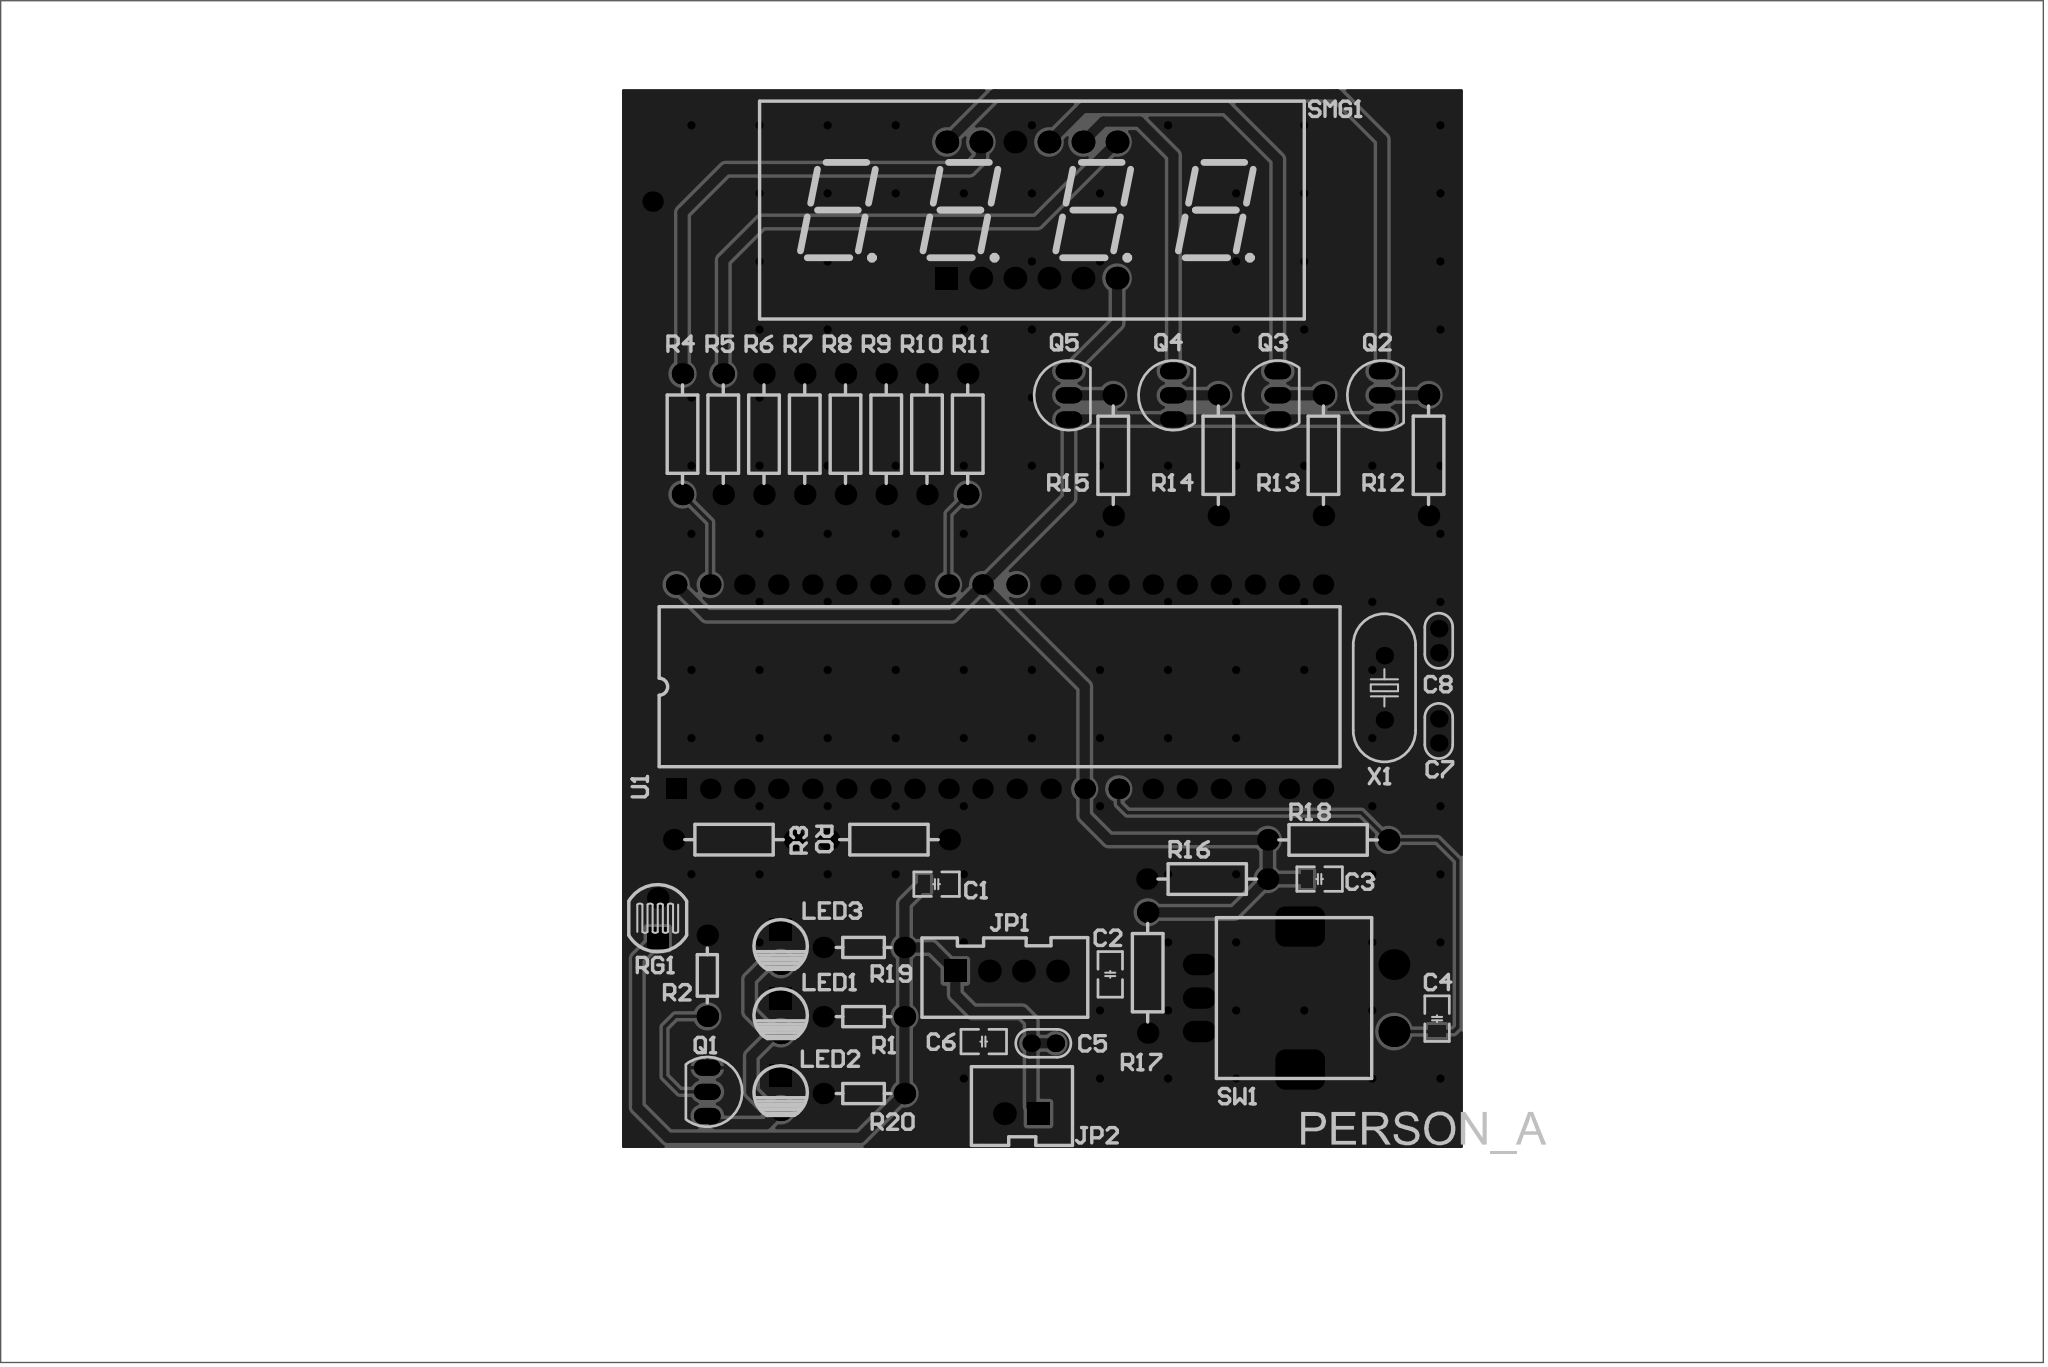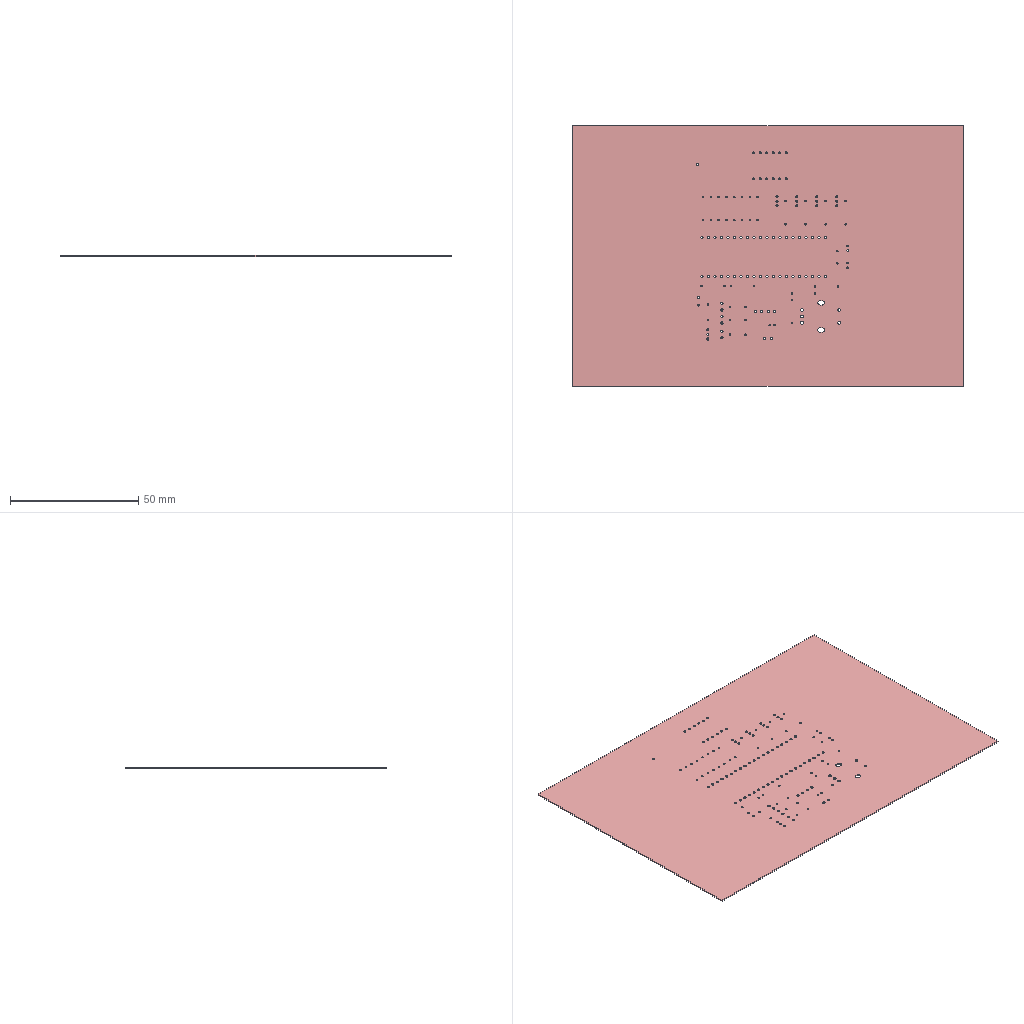Circuit board layout | Altium Designer | box 152.4 x 101.6 x 0.4 mm
Layer stack:
# Altium Designer layer stack of  (unit mm; dielectric type: 0 none, 1 core, 2 prepreg, 3 surface material)
index,name,kind,layer,copper_thickness_mm,dielectric_type,dielectric_thickness_mm,dielectric_material,dielectric_constant
0,Top Paste Mask Layer,other,,,,,,
1,Top Silkscreen Layer,other,,,,,,
2,Top Solder Mask Layer,dielectric,,,3,0.0102,Solder Resist,3.5
3,Top Layer,copper,Top Layer,0.0356,,,,
4,Dielectric 1,dielectric,,,3,0.32,FR-4,4.8
5,Bottom Layer,copper,Bottom Layer,0.0356,,,,
6,Bottom Solder Mask Layer,dielectric,,,3,0.0102,Solder Resist,3.5
7,Bottom Silkscreen Layer,other,,,,,,
8,Bottom Paste Mask Layer,other,,,,,,
# drill layer pairs: low layer,high layer
drill_pair,Top Layer,Bottom Layer
Part placement:
Designator,Comment,Layer,Footprint,Center-X(mm),Center-Y(mm),Rotation
X1,11.059MHz,TopLayer,HC-49S,179.438,126.536,270
U1,STC12C5A60S2,TopLayer,DIP-40,150.729,126.619,90
SW1,EC11,TopLayer,EC11-B,172.903,103.391,180
SMG1,4041B,TopLayer,SMG_0.4-4P,153.142,162.179,0
RG1,10K,TopLayer,RG5528,125.222,109.347,90
R20,100,TopLayer,AXIAL0.3-1/8W,140.604,96.266,0
R19,100,TopLayer,AXIAL0.3-1/8W,140.604,107.165,0
R18,10K,TopLayer,AXIAL0.4-1/4W,175.24,115.189,180
R17,10K,TopLayer,AXIAL0.4-1/4W,161.778,105.283,270
R16,10K,TopLayer,AXIAL0.4-1/4W,166.223,112.268,0
R15,1K,TopLayer,AXIAL0.4-1/4W,159.208,143.887,90
R14,1K,TopLayer,AXIAL0.4-1/4W,167.049,143.887,90
R13,1K,TopLayer,AXIAL0.4-1/4W,174.891,143.887,90
R12,1K,TopLayer,AXIAL0.4-1/4W,182.733,143.887,90
R11,220,TopLayer,AXIAL0.4-1/4W,148.351,145.462,90
R10,220,TopLayer,AXIAL0.4-1/4W,145.311,145.462,270
R9,220,TopLayer,AXIAL0.4-1/4W,142.271,145.462,90
R8,220,TopLayer,AXIAL0.4-1/4W,139.231,145.462,90
R7,220,TopLayer,AXIAL0.4-1/4W,136.191,145.462,90
R6,220,TopLayer,AXIAL0.4-1/4W,133.151,145.462,90
R5,220,TopLayer,AXIAL0.4-1/4W,130.111,145.462,90
R4,220,TopLayer,AXIAL0.4-1/4W,127.071,145.462,270
R3,10K,TopLayer,AXIAL0.4-1/4W,142.474,115.209,180
R2,1K,TopLayer,AXIAL0.3-1/8W,128.922,105.053,270
R1,100,TopLayer,AXIAL0.3-1/8W,140.604,102.004,0
R0,10K,TopLayer,AXIAL0.4-1/4W,130.917,115.209,0
Q5,S9012,TopLayer,TO92A,155.906,148.357,90
Q4,S9012,TopLayer,TO92A,163.695,148.357,90
Q3,S9012,TopLayer,TO92A,171.484,148.357,90
Q2,S9012,TopLayer,TO92A,179.274,148.357,90
Q1,S9013,TopLayer,TO92A,128.922,96.393,270
LED3,Red,TopLayer,LED_3MM-B,134.405,107.233,270
LED2,Red,TopLayer,LED_3MM-B,134.405,96.334,270
LED1,Red,TopLayer,LED_3MM-B,134.405,102.072,270
JP2,HDR-1X2,TopLayer,XH2.54-LI-2P,152.361,94.766,180
JP1,HDR-1X4,TopLayer,XH2.54-LI-4P,151.237,105.41,0
C8,22pF,TopLayer,CC_1.8*3.6,183.495,130.048,270
C7,22pF,TopLayer,CC_1.8*3.6,183.495,123.317,90
C6,220uF,TopLayer,C0805_L,149.546,100.142,180
C5,104,TopLayer,CC_1.8*3.6,153.991,100.015,0
C4,0.1uF,TopLayer,C0805_L,183.368,101.854,270
C3,0.1uF,TopLayer,C0805_L,174.605,112.268,0
C2,0.1uF,TopLayer,C0805_L,158.984,105.156,90
C1,10uF,TopLayer,C0805_L,146.03,111.887,180
Pad and via stacks:
# Altium Designer via and pad stacks of  (unit mm). Each distinct definition once, with the count of objects using it.
# via: kind,start_layer,end_layer,hole_mm,diameter_mm,mode(0 simple;1 top-mid-bottom;2 full stack),diameter_per_layer,count,example_net
# pad: kind,layer,hole_mm,hole_type(0 round;1 square;2 slot),plating,top_size,top_shape(1 round;2 rect;3 octagon;9 rounded rect),mid_size,bottom_size,mode,footprint,size_per_layer,count,example
pad,Multi-Layer,0.6,0,plated,1.3x1.3,1,1.3x1.3,1.3x1.3,0,HC-49S,,2,X1.1
pad,Multi-Layer,0.889,0,plated,1.524x1.524,2,1.524x1.524,1.524x1.524,0,DIP-40,,1,U1.1
pad,Multi-Layer,0.889,0,plated,1.524x1.524,1,1.524x1.524,1.524x1.524,0,DIP-40,,39,U1.2
pad,Multi-Layer,1.8,2,plated,3x3.7,9,3x3.7,3x3.7,0,EC11-B,,2,SW1.0
pad,Multi-Layer,1.1,0,plated,2.3x2.3,1,2.3x2.3,2.3x2.3,0,EC11-B,,2,SW1.2
pad,Multi-Layer,1.1,0,plated,1.6x2.5,1,1.6x2.5,1.6x2.5,0,EC11-B,,3,SW1.B
pad,Multi-Layer,0.8,0,plated,1.7x1.7,2,1.7x1.7,1.7x1.7,0,SMG 0.4-4P,,1,SMG1.1
pad,Multi-Layer,0.8,0,plated,1.7x1.7,1,1.7x1.7,1.7x1.7,0,SMG 0.4-4P,,11,SMG1.2
pad,Multi-Layer,0.8,0,plated,1.6x1.6,1,1.6x1.6,1.6x1.6,0,RG5528,,1,RG1.2
pad,Multi-Layer,0.8,0,plated,1.6x1.6,2,1.6x1.6,1.6x1.6,0,RG5528,,1,RG1.1
pad,Multi-Layer,0.6,0,plated,1.6x1.6,1,1.6x1.6,1.6x1.6,0,AXIAL0.3-1/8W,,8,R20.2
pad,Multi-Layer,0.6,0,plated,1.6x1.6,1,1.6x1.6,1.6x1.6,0,AXIAL0.4-1/4W,,34,R18.2
pad,Multi-Layer,0.8,0,plated,2x1.2,1,2x1.2,2x1.2,0,TO92A,,15,Q5.3
pad,Multi-Layer,0.9,0,plated,1.7x1.7,2,1.7x1.7,1.7x1.7,0,LED 3MM-B,,3,LED3.1
pad,Multi-Layer,0.9,0,plated,1.7x1.7,1,1.7x1.7,1.7x1.7,0,LED 3MM-B,,3,LED3.2
pad,Multi-Layer,0.9,0,plated,1.7x1.7,1,1.7x1.7,1.7x1.7,0,XH2.54-LI-2P,,1,JP2.2
pad,Multi-Layer,0.9,0,plated,1.7x1.7,2,1.7x1.7,1.7x1.7,0,XH2.54-LI-2P,,1,JP2.1
pad,Multi-Layer,0.9,0,plated,1.7x1.7,1,1.7x1.7,1.7x1.7,0,XH2.54-LI-4P,,3,JP1.4
pad,Multi-Layer,0.9,0,plated,1.7x1.7,2,1.7x1.7,1.7x1.7,0,XH2.54-LI-4P,,1,JP1.1
pad,Multi-Layer,0.635,0,plated,1.3x1.3,1,1.3x1.3,1.3x1.3,0,CC 1.8*3.6,,6,C8.2
pad,Multi-Layer,0.9144,0,plated,1.524x1.524,1,1.524x1.524,1.524x1.524,0,,,1,1
pad,Top Layer,0,0,plated,1.27x0.889,2,1.27x0.889,1.27x0.889,0,C0805_L,,10,C6.2
via,Top Layer,Bottom Layer,0.3048,0.6096,0,,117,GND
Copper pours:
name,layer,net,type(0 solid;1 hatched;2 none)
Top Layer-GND,Top Layer,GND,0
Bottom Layer-GND,Bottom Layer,GND,0
Design rules, without the lines most boards share:
# Altium Designer design rules of  (exported by Altium Designer, unit mm)
# columns: name | kind | enabled | priority | scope1 | scope2 | descriptor | typed fields (field=value)
ComponentClearance_1 | 24 | enabled | 1 | All | All | Component Clearance Constraint ( Horizontal Gap = 10mil, Vertical Gap = 10mil ) (All),(All)  | gap=0.254
Clearance | 0 | enabled | 1 | All | All | Clearance Constraint (Gap=10mil) (All),(All) | gap=0.254
Clearance_1 | 63 | enabled | 1 | All | All | Board Clearance Constraint (Gap=0mil) (All) |
ComponentClearance | 52 | enabled | 1 | All | All | Hole To Hole Clearance (Gap=10mil) (All),(All) | gap=0.254
Width | 2 | enabled | 1 | All | All | Width Constraint (Min=10mil) (Max=17952.8mil) (Preferred=10mil) (All) |
DiffPairsRouting | 51 | enabled | 1 | All | All | Differential Pairs Uncoupled Length using the Gap Constraints (Min=10mil) (Max=10mil) (Prefered=10mil)  and Width Constraints (Min=15mil) (Max=15mil) (Prefered=15mil) (All) |
RoutingVias | 11 | enabled | 1 | All | All | Routing Via (MinHoleWidth=1mil) (MaxHoleWidth=28mil) (PreferredHoleWidth=28mil) (MinWidth=1mil) (MaxWidth=50mil) (PreferedWidth=50mil) (All) | via_min_hole=0.0254 via_max_hole=0.7112 via_preferred_diameter=1.27 via_preferred_hole=0.7112
PlaneConnect | 6 | enabled | 1 | All | All | Power Plane Connect Rule(Relief Connect )(Expansion=20mil) (Conductor Width=10mil) (Air Gap=10mil) (Entries=4) (All) | relief_conductor_width=0.254 relief_entries=4 relief_expansion=0.508
PolygonConnect | 20 | enabled | 1 | (InNet('GND')) | All | Polygon Connect Rule(Relief Connect )(Conductor Width=10mil) (Relief Angle=90 Angle) (Entries=4) (Air Gap Width=10mil) ((InNet('GND'))),(All) | connect_style(0=relief,1=direct,2=none)=0 relief_conductor_width=0.254 relief_entries=4
PasteMaskExpansion | 14 | enabled | 1 | All | All | Paste Mask Expansion (Expansion =0mil) (All) | expansion=0
SolderMaskExpansion | 13 | enabled | 1 | All | All | Solder Mask Expansion (Expansion =4mil) (All) | expansion=0.1016